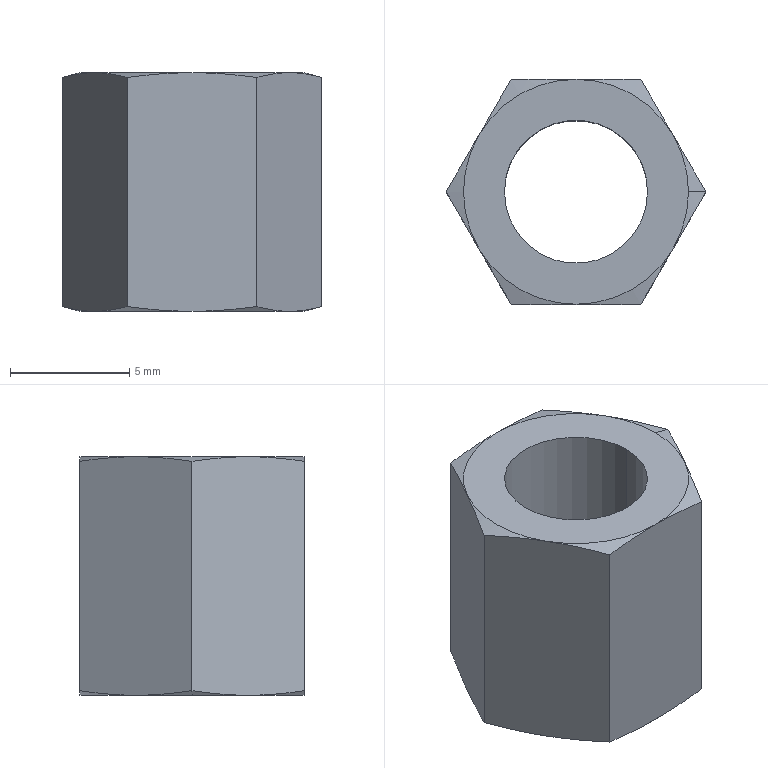Part | SolidWorks | features Cut 2, Chamfer 1, Extrusion 1, MoveFace 1 | 1 solid | 24 faces | box 10.89 x 9.431 x 10 mm | volume 486.676 mm3 | cone 14 | plane 8 | cylinder 2 | commonest cylinder face diameters 6 x2
STEP:
#1=CARTESIAN_POINT('',(4.716,0.,6.4));
#2=VERTEX_POINT('',#1);
#3=CARTESIAN_POINT('',(4.084,2.358,6.4));
#4=VERTEX_POINT('',#3);
#5=CARTESIAN_POINT('',(0.,0.,6.4));
#6=DIRECTION('',(0.,0.,1.));
#7=DIRECTION('',(1.,0.,0.));
#8=AXIS2_PLACEMENT_3D('',#5,#6,#7);
#9=CIRCLE('',#8,4.716);
#10=EDGE_CURVE('',#2,#4,#9,.T.);
#11=ORIENTED_EDGE('',*,*,#10,.F.);
#12=CARTESIAN_POINT('',(5.445,0.,6.205));
#13=VERTEX_POINT('',#12);
#14=CARTESIAN_POINT('',(4.716,0.,6.4));
#15=DIRECTION('',(0.9659,0.,-0.2588));
#16=VECTOR('',#15,1000.);
#17=LINE('',#14,#16);
#18=EDGE_CURVE('',#2,#13,#17,.T.);
#19=ORIENTED_EDGE('',*,*,#18,.T.);
#20=CARTESIAN_POINT('',(5.445,0.,6.205));
#21=CARTESIAN_POINT('',(4.991,0.7859,6.326));
#22=CARTESIAN_POINT('',(4.538,1.572,6.4));
#23=CARTESIAN_POINT('',(4.084,2.358,6.4));
#24=B_SPLINE_CURVE_WITH_KNOTS('',3,(#20,#21,#22,#23),.UNSPECIFIED.,.F.,.F.,(4,4),(0.000000231,0.002723),.UNSPECIFIED.);
#25=EDGE_CURVE('',#13,#4,#24,.T.);
#26=ORIENTED_EDGE('',*,*,#25,.T.);
#27=EDGE_LOOP('',(#11,#19,#26));
#28=FACE_OUTER_BOUND('',#27,.T.);
#29=CARTESIAN_POINT('',(0.,0.,6.4));
#30=DIRECTION('',(0.,0.,-1.));
#31=DIRECTION('',(1.,0.,0.));
#32=AXIS2_PLACEMENT_3D('',#29,#30,#31);
#33=CONICAL_SURFACE('',#32,4.716,1.309);
#34=ADVANCED_FACE('',(#28),#33,.T.);
#35=CARTESIAN_POINT('',(-4.716,0.,-3.6));
#36=VERTEX_POINT('',#35);
#37=CARTESIAN_POINT('',(-4.084,2.358,-3.6));
#38=VERTEX_POINT('',#37);
#39=CARTESIAN_POINT('',(0.,0.,-3.6));
#40=DIRECTION('',(0.,0.,-1.));
#41=DIRECTION('',(-1.,0.,0.));
#42=AXIS2_PLACEMENT_3D('',#39,#40,#41);
#43=CIRCLE('',#42,4.716);
#44=EDGE_CURVE('',#36,#38,#43,.T.);
#45=ORIENTED_EDGE('',*,*,#44,.F.);
#46=CARTESIAN_POINT('',(-5.445,0.,-3.405));
#47=VERTEX_POINT('',#46);
#48=CARTESIAN_POINT('',(-4.716,0.,-3.6));
#49=DIRECTION('',(-0.9659,0.,0.2588));
#50=VECTOR('',#49,1000.);
#51=LINE('',#48,#50);
#52=EDGE_CURVE('',#36,#47,#51,.T.);
#53=ORIENTED_EDGE('',*,*,#52,.T.);
#54=CARTESIAN_POINT('',(-5.445,0.,-3.405));
#55=CARTESIAN_POINT('',(-4.991,0.7861,-3.526));
#56=CARTESIAN_POINT('',(-4.537,1.572,-3.6));
#57=CARTESIAN_POINT('',(-4.084,2.358,-3.6));
#58=B_SPLINE_CURVE_WITH_KNOTS('',3,(#54,#55,#56,#57),.UNSPECIFIED.,.F.,.F.,(4,4),(0.02771,0.03044),.UNSPECIFIED.);
#59=EDGE_CURVE('',#47,#38,#58,.T.);
#60=ORIENTED_EDGE('',*,*,#59,.T.);
#61=EDGE_LOOP('',(#45,#53,#60));
#62=FACE_OUTER_BOUND('',#61,.T.);
#63=CARTESIAN_POINT('',(0.,0.,-3.6));
#64=DIRECTION('',(0.,0.,1.));
#65=DIRECTION('',(-1.,0.,0.));
#66=AXIS2_PLACEMENT_3D('',#63,#64,#65);
#67=CONICAL_SURFACE('',#66,4.716,1.309);
#68=ADVANCED_FACE('',(#62),#67,.T.);
#69=CARTESIAN_POINT('',(-3.,0.,6.4));
#70=VERTEX_POINT('',#69);
#71=CARTESIAN_POINT('',(3.,0.,6.4));
#72=VERTEX_POINT('',#71);
#73=CARTESIAN_POINT('',(0.,0.,6.4));
#74=DIRECTION('',(0.,0.,1.));
#75=DIRECTION('',(1.,0.,0.));
#76=AXIS2_PLACEMENT_3D('',#73,#74,#75);
#77=CIRCLE('',#76,3.);
#78=EDGE_CURVE('',#70,#72,#77,.T.);
#79=ORIENTED_EDGE('',*,*,#78,.T.);
#80=CARTESIAN_POINT('',(3.,0.,-3.6));
#81=VERTEX_POINT('',#80);
#82=CARTESIAN_POINT('',(3.,0.,6.4));
#83=DIRECTION('',(0.,0.,-1.));
#84=VECTOR('',#83,1000.);
#85=LINE('',#82,#84);
#86=EDGE_CURVE('',#72,#81,#85,.T.);
#87=ORIENTED_EDGE('',*,*,#86,.T.);
#88=CARTESIAN_POINT('',(-3.,0.,-3.6));
#89=VERTEX_POINT('',#88);
#90=CARTESIAN_POINT('',(0.,0.,-3.6));
#91=DIRECTION('',(0.,0.,1.));
#92=DIRECTION('',(1.,0.,0.));
#93=AXIS2_PLACEMENT_3D('',#90,#91,#92);
#94=CIRCLE('',#93,3.);
#95=EDGE_CURVE('',#89,#81,#94,.T.);
#96=ORIENTED_EDGE('',*,*,#95,.F.);
#97=CARTESIAN_POINT('',(-3.,0.,6.4));
#98=DIRECTION('',(0.,0.,-1.));
#99=VECTOR('',#98,1000.);
#100=LINE('',#97,#99);
#101=EDGE_CURVE('',#70,#89,#100,.T.);
#102=ORIENTED_EDGE('',*,*,#101,.F.);
#103=EDGE_LOOP('',(#79,#87,#96,#102));
#104=FACE_OUTER_BOUND('',#103,.T.);
#105=CARTESIAN_POINT('',(0.,0.,6.4));
#106=DIRECTION('',(0.,0.,-1.));
#107=DIRECTION('',(-1.,0.,0.));
#108=AXIS2_PLACEMENT_3D('',#105,#106,#107);
#109=CYLINDRICAL_SURFACE('',#108,3.);
#110=ADVANCED_FACE('',(#104),#109,.F.);
#111=ORIENTED_EDGE('',*,*,#25,.F.);
#112=CARTESIAN_POINT('',(5.445,0.,-3.405));
#113=VERTEX_POINT('',#112);
#114=CARTESIAN_POINT('',(5.445,0.,6.4));
#115=DIRECTION('',(0.,0.,-1.));
#116=VECTOR('',#115,1000.);
#117=LINE('',#114,#116);
#118=EDGE_CURVE('',#13,#113,#117,.T.);
#119=ORIENTED_EDGE('',*,*,#118,.T.);
#120=CARTESIAN_POINT('',(4.084,2.358,-3.6));
#121=VERTEX_POINT('',#120);
#122=CARTESIAN_POINT('',(4.084,2.358,-3.6));
#123=CARTESIAN_POINT('',(4.311,1.965,-3.6));
#124=CARTESIAN_POINT('',(4.539,1.569,-3.582));
#125=CARTESIAN_POINT('',(4.993,0.7831,-3.514));
#126=CARTESIAN_POINT('',(5.219,0.3911,-3.465));
#127=CARTESIAN_POINT('',(5.445,0.,-3.405));
#128=B_SPLINE_CURVE_WITH_KNOTS('',3,(#122,#123,#124,#125,#126,#127),.UNSPECIFIED.,.F.,.F.,(4,2,4),(0.02511,0.02644,0.02777),.UNSPECIFIED.);
#129=EDGE_CURVE('',#121,#113,#128,.T.);
#130=ORIENTED_EDGE('',*,*,#129,.F.);
#131=CARTESIAN_POINT('',(2.723,4.716,-3.405));
#132=VERTEX_POINT('',#131);
#133=CARTESIAN_POINT('',(2.723,4.716,-3.405));
#134=CARTESIAN_POINT('',(3.176,3.929,-3.526));
#135=CARTESIAN_POINT('',(3.63,3.143,-3.6));
#136=CARTESIAN_POINT('',(4.084,2.358,-3.6));
#137=B_SPLINE_CURVE_WITH_KNOTS('',3,(#133,#134,#135,#136),.UNSPECIFIED.,.F.,.F.,(4,4),(0.02771,0.03044),.UNSPECIFIED.);
#138=EDGE_CURVE('',#132,#121,#137,.T.);
#139=ORIENTED_EDGE('',*,*,#138,.F.);
#140=CARTESIAN_POINT('',(2.723,4.716,6.205));
#141=VERTEX_POINT('',#140);
#142=CARTESIAN_POINT('',(2.723,4.716,6.4));
#143=DIRECTION('',(0.,0.,-1.));
#144=VECTOR('',#143,1000.);
#145=LINE('',#142,#144);
#146=EDGE_CURVE('',#141,#132,#145,.T.);
#147=ORIENTED_EDGE('',*,*,#146,.F.);
#148=CARTESIAN_POINT('',(4.084,2.358,6.4));
#149=CARTESIAN_POINT('',(3.63,3.144,6.4));
#150=CARTESIAN_POINT('',(3.176,3.93,6.326));
#151=CARTESIAN_POINT('',(2.723,4.716,6.205));
#152=B_SPLINE_CURVE_WITH_KNOTS('',3,(#148,#149,#150,#151),.UNSPECIFIED.,.F.,.F.,(4,4),(0.002723,0.005445),.UNSPECIFIED.);
#153=EDGE_CURVE('',#4,#141,#152,.T.);
#154=ORIENTED_EDGE('',*,*,#153,.F.);
#155=EDGE_LOOP('',(#111,#119,#130,#139,#147,#154));
#156=FACE_OUTER_BOUND('',#155,.T.);
#157=CARTESIAN_POINT('',(5.445,0.,6.4));
#158=DIRECTION('',(-0.866,-0.5,0.));
#159=DIRECTION('',(0.5,-0.866,0.));
#160=AXIS2_PLACEMENT_3D('',#157,#158,#159);
#161=PLANE('',#160);
#162=ADVANCED_FACE('',(#156),#161,.F.);
#163=CARTESIAN_POINT('',(0.,4.716,6.4));
#164=VERTEX_POINT('',#163);
#165=CARTESIAN_POINT('',(2.723,4.716,6.205));
#166=CARTESIAN_POINT('',(1.816,4.716,6.326));
#167=CARTESIAN_POINT('',(0.9092,4.716,6.4));
#168=CARTESIAN_POINT('',(0.,4.716,6.4));
#169=B_SPLINE_CURVE_WITH_KNOTS('',3,(#165,#166,#167,#168),.UNSPECIFIED.,.F.,.F.,(4,4),(0.01615,0.01889),.UNSPECIFIED.);
#170=EDGE_CURVE('',#141,#164,#169,.T.);
#171=ORIENTED_EDGE('',*,*,#170,.F.);
#172=ORIENTED_EDGE('',*,*,#146,.T.);
#173=CARTESIAN_POINT('',(0.,4.716,-3.6));
#174=VERTEX_POINT('',#173);
#175=CARTESIAN_POINT('',(0.,4.716,-3.6));
#176=CARTESIAN_POINT('',(0.454,4.716,-3.6));
#177=CARTESIAN_POINT('',(0.9107,4.716,-3.582));
#178=CARTESIAN_POINT('',(1.818,4.716,-3.514));
#179=CARTESIAN_POINT('',(2.271,4.716,-3.465));
#180=CARTESIAN_POINT('',(2.723,4.716,-3.405));
#181=B_SPLINE_CURVE_WITH_KNOTS('',3,(#175,#176,#177,#178,#179,#180),.UNSPECIFIED.,.F.,.F.,(4,2,4),(0.02511,0.02644,0.02777),.UNSPECIFIED.);
#182=EDGE_CURVE('',#174,#132,#181,.T.);
#183=ORIENTED_EDGE('',*,*,#182,.F.);
#184=CARTESIAN_POINT('',(-2.722,4.716,-3.405));
#185=VERTEX_POINT('',#184);
#186=CARTESIAN_POINT('',(-2.722,4.716,-3.405));
#187=CARTESIAN_POINT('',(-1.815,4.716,-3.526));
#188=CARTESIAN_POINT('',(-0.9073,4.716,-3.6));
#189=CARTESIAN_POINT('',(0.,4.716,-3.6));
#190=B_SPLINE_CURVE_WITH_KNOTS('',3,(#186,#187,#188,#189),.UNSPECIFIED.,.F.,.F.,(4,4),(0.02771,0.03044),.UNSPECIFIED.);
#191=EDGE_CURVE('',#185,#174,#190,.T.);
#192=ORIENTED_EDGE('',*,*,#191,.F.);
#193=CARTESIAN_POINT('',(-2.722,4.716,6.205));
#194=VERTEX_POINT('',#193);
#195=CARTESIAN_POINT('',(-2.722,4.716,6.4));
#196=DIRECTION('',(0.,0.,-1.));
#197=VECTOR('',#196,1000.);
#198=LINE('',#195,#197);
#199=EDGE_CURVE('',#194,#185,#198,.T.);
#200=ORIENTED_EDGE('',*,*,#199,.F.);
#201=CARTESIAN_POINT('',(0.,4.716,6.4));
#202=CARTESIAN_POINT('',(-0.4531,4.716,6.4));
#203=CARTESIAN_POINT('',(-0.9068,4.716,6.382));
#204=CARTESIAN_POINT('',(-1.815,4.716,6.315));
#205=CARTESIAN_POINT('',(-2.27,4.716,6.265));
#206=CARTESIAN_POINT('',(-2.722,4.716,6.205));
#207=B_SPLINE_CURVE_WITH_KNOTS('',3,(#201,#202,#203,#204,#205,#206),.UNSPECIFIED.,.F.,.F.,(4,2,4),(0.01889,0.02026,0.02162),.UNSPECIFIED.);
#208=EDGE_CURVE('',#164,#194,#207,.T.);
#209=ORIENTED_EDGE('',*,*,#208,.F.);
#210=EDGE_LOOP('',(#171,#172,#183,#192,#200,#209));
#211=FACE_OUTER_BOUND('',#210,.T.);
#212=CARTESIAN_POINT('',(2.723,4.716,6.4));
#213=DIRECTION('',(0.,-1.,0.));
#214=DIRECTION('',(0.,0.,-1.));
#215=AXIS2_PLACEMENT_3D('',#212,#213,#214);
#216=PLANE('',#215);
#217=ADVANCED_FACE('',(#211),#216,.F.);
#218=CARTESIAN_POINT('',(-4.084,2.358,6.4));
#219=VERTEX_POINT('',#218);
#220=CARTESIAN_POINT('',(-2.722,4.716,6.205));
#221=CARTESIAN_POINT('',(-3.176,3.93,6.326));
#222=CARTESIAN_POINT('',(-3.63,3.144,6.4));
#223=CARTESIAN_POINT('',(-4.084,2.358,6.4));
#224=B_SPLINE_CURVE_WITH_KNOTS('',3,(#220,#221,#222,#223),.UNSPECIFIED.,.F.,.F.,(4,4),(0.000000231,0.002723),.UNSPECIFIED.);
#225=EDGE_CURVE('',#194,#219,#224,.T.);
#226=ORIENTED_EDGE('',*,*,#225,.F.);
#227=ORIENTED_EDGE('',*,*,#199,.T.);
#228=CARTESIAN_POINT('',(-4.084,2.358,-3.6));
#229=CARTESIAN_POINT('',(-3.857,2.751,-3.6));
#230=CARTESIAN_POINT('',(-3.628,3.146,-3.582));
#231=CARTESIAN_POINT('',(-3.175,3.932,-3.514));
#232=CARTESIAN_POINT('',(-2.948,4.324,-3.465));
#233=CARTESIAN_POINT('',(-2.722,4.716,-3.405));
#234=B_SPLINE_CURVE_WITH_KNOTS('',3,(#228,#229,#230,#231,#232,#233),.UNSPECIFIED.,.F.,.F.,(4,2,4),(0.02511,0.02644,0.02777),.UNSPECIFIED.);
#235=EDGE_CURVE('',#38,#185,#234,.T.);
#236=ORIENTED_EDGE('',*,*,#235,.F.);
#237=ORIENTED_EDGE('',*,*,#59,.F.);
#238=CARTESIAN_POINT('',(-5.445,0.,6.205));
#239=VERTEX_POINT('',#238);
#240=CARTESIAN_POINT('',(-5.445,0.,6.4));
#241=DIRECTION('',(0.,0.,-1.));
#242=VECTOR('',#241,1000.);
#243=LINE('',#240,#242);
#244=EDGE_CURVE('',#239,#47,#243,.T.);
#245=ORIENTED_EDGE('',*,*,#244,.F.);
#246=CARTESIAN_POINT('',(-4.084,2.358,6.4));
#247=CARTESIAN_POINT('',(-4.537,1.572,6.4));
#248=CARTESIAN_POINT('',(-4.991,0.7859,6.326));
#249=CARTESIAN_POINT('',(-5.445,0.,6.205));
#250=B_SPLINE_CURVE_WITH_KNOTS('',3,(#246,#247,#248,#249),.UNSPECIFIED.,.F.,.F.,(4,4),(0.002723,0.005445),.UNSPECIFIED.);
#251=EDGE_CURVE('',#219,#239,#250,.T.);
#252=ORIENTED_EDGE('',*,*,#251,.F.);
#253=EDGE_LOOP('',(#226,#227,#236,#237,#245,#252));
#254=FACE_OUTER_BOUND('',#253,.T.);
#255=CARTESIAN_POINT('',(-2.722,4.716,6.4));
#256=DIRECTION('',(0.866,-0.5,0.));
#257=DIRECTION('',(0.5,0.866,0.));
#258=AXIS2_PLACEMENT_3D('',#255,#256,#257);
#259=PLANE('',#258);
#260=ADVANCED_FACE('',(#254),#259,.F.);
#261=CARTESIAN_POINT('',(-4.084,-2.358,6.4));
#262=VERTEX_POINT('',#261);
#263=CARTESIAN_POINT('',(-5.445,0.,6.205));
#264=CARTESIAN_POINT('',(-4.991,-0.7859,6.326));
#265=CARTESIAN_POINT('',(-4.537,-1.572,6.4));
#266=CARTESIAN_POINT('',(-4.084,-2.358,6.4));
#267=B_SPLINE_CURVE_WITH_KNOTS('',3,(#263,#264,#265,#266),.UNSPECIFIED.,.F.,.F.,(4,4),(0.000000231,0.002723),.UNSPECIFIED.);
#268=EDGE_CURVE('',#239,#262,#267,.T.);
#269=ORIENTED_EDGE('',*,*,#268,.F.);
#270=ORIENTED_EDGE('',*,*,#244,.T.);
#271=CARTESIAN_POINT('',(-4.084,-2.358,-3.6));
#272=VERTEX_POINT('',#271);
#273=CARTESIAN_POINT('',(-4.084,-2.358,-3.6));
#274=CARTESIAN_POINT('',(-4.311,-1.965,-3.6));
#275=CARTESIAN_POINT('',(-4.539,-1.569,-3.582));
#276=CARTESIAN_POINT('',(-4.993,-0.7831,-3.514));
#277=CARTESIAN_POINT('',(-5.219,-0.3911,-3.465));
#278=CARTESIAN_POINT('',(-5.445,0.,-3.405));
#279=B_SPLINE_CURVE_WITH_KNOTS('',3,(#273,#274,#275,#276,#277,#278),.UNSPECIFIED.,.F.,.F.,(4,2,4),(0.02511,0.02644,0.02777),.UNSPECIFIED.);
#280=EDGE_CURVE('',#272,#47,#279,.T.);
#281=ORIENTED_EDGE('',*,*,#280,.F.);
#282=CARTESIAN_POINT('',(-2.722,-4.716,-3.405));
#283=VERTEX_POINT('',#282);
#284=CARTESIAN_POINT('',(-2.722,-4.716,-3.405));
#285=CARTESIAN_POINT('',(-3.176,-3.929,-3.526));
#286=CARTESIAN_POINT('',(-3.63,-3.143,-3.6));
#287=CARTESIAN_POINT('',(-4.084,-2.358,-3.6));
#288=B_SPLINE_CURVE_WITH_KNOTS('',3,(#284,#285,#286,#287),.UNSPECIFIED.,.F.,.F.,(4,4),(0.02771,0.03044),.UNSPECIFIED.);
#289=EDGE_CURVE('',#283,#272,#288,.T.);
#290=ORIENTED_EDGE('',*,*,#289,.F.);
#291=CARTESIAN_POINT('',(-2.722,-4.716,6.205));
#292=VERTEX_POINT('',#291);
#293=CARTESIAN_POINT('',(-2.722,-4.716,6.4));
#294=DIRECTION('',(0.,0.,-1.));
#295=VECTOR('',#294,1000.);
#296=LINE('',#293,#295);
#297=EDGE_CURVE('',#292,#283,#296,.T.);
#298=ORIENTED_EDGE('',*,*,#297,.F.);
#299=CARTESIAN_POINT('',(-4.084,-2.358,6.4));
#300=CARTESIAN_POINT('',(-3.63,-3.144,6.4));
#301=CARTESIAN_POINT('',(-3.176,-3.93,6.326));
#302=CARTESIAN_POINT('',(-2.722,-4.716,6.205));
#303=B_SPLINE_CURVE_WITH_KNOTS('',3,(#299,#300,#301,#302),.UNSPECIFIED.,.F.,.F.,(4,4),(0.002723,0.005445),.UNSPECIFIED.);
#304=EDGE_CURVE('',#262,#292,#303,.T.);
#305=ORIENTED_EDGE('',*,*,#304,.F.);
#306=EDGE_LOOP('',(#269,#270,#281,#290,#298,#305));
#307=FACE_OUTER_BOUND('',#306,.T.);
#308=CARTESIAN_POINT('',(-5.445,0.,6.4));
#309=DIRECTION('',(0.866,0.5,0.));
#310=DIRECTION('',(-0.5,0.866,0.));
#311=AXIS2_PLACEMENT_3D('',#308,#309,#310);
#312=PLANE('',#311);
#313=ADVANCED_FACE('',(#307),#312,.F.);
#314=CARTESIAN_POINT('',(0.,-4.716,6.4));
#315=VERTEX_POINT('',#314);
#316=CARTESIAN_POINT('',(-2.722,-4.716,6.205));
#317=CARTESIAN_POINT('',(-2.27,-4.716,6.265));
#318=CARTESIAN_POINT('',(-1.815,-4.716,6.315));
#319=CARTESIAN_POINT('',(-0.9068,-4.716,6.382));
#320=CARTESIAN_POINT('',(-0.4531,-4.716,6.4));
#321=CARTESIAN_POINT('',(0.,-4.716,6.4));
#322=B_SPLINE_CURVE_WITH_KNOTS('',3,(#316,#317,#318,#319,#320,#321),.UNSPECIFIED.,.F.,.F.,(4,2,4),(0.004659,0.006027,0.007395),.UNSPECIFIED.);
#323=EDGE_CURVE('',#292,#315,#322,.T.);
#324=ORIENTED_EDGE('',*,*,#323,.F.);
#325=ORIENTED_EDGE('',*,*,#297,.T.);
#326=CARTESIAN_POINT('',(0.,-4.716,-3.6));
#327=VERTEX_POINT('',#326);
#328=CARTESIAN_POINT('',(0.,-4.716,-3.6));
#329=CARTESIAN_POINT('',(-0.454,-4.716,-3.6));
#330=CARTESIAN_POINT('',(-0.9107,-4.716,-3.582));
#331=CARTESIAN_POINT('',(-1.818,-4.716,-3.514));
#332=CARTESIAN_POINT('',(-2.271,-4.716,-3.465));
#333=CARTESIAN_POINT('',(-2.722,-4.716,-3.405));
#334=B_SPLINE_CURVE_WITH_KNOTS('',3,(#328,#329,#330,#331,#332,#333),.UNSPECIFIED.,.F.,.F.,(4,2,4),(0.02511,0.02644,0.02777),.UNSPECIFIED.);
#335=EDGE_CURVE('',#327,#283,#334,.T.);
#336=ORIENTED_EDGE('',*,*,#335,.F.);
#337=CARTESIAN_POINT('',(2.723,-4.716,-3.405));
#338=VERTEX_POINT('',#337);
#339=CARTESIAN_POINT('',(2.723,-4.716,-3.405));
#340=CARTESIAN_POINT('',(1.815,-4.716,-3.526));
#341=CARTESIAN_POINT('',(0.9073,-4.716,-3.6));
#342=CARTESIAN_POINT('',(0.,-4.716,-3.6));
#343=B_SPLINE_CURVE_WITH_KNOTS('',3,(#339,#340,#341,#342),.UNSPECIFIED.,.F.,.F.,(4,4),(0.02771,0.03044),.UNSPECIFIED.);
#344=EDGE_CURVE('',#338,#327,#343,.T.);
#345=ORIENTED_EDGE('',*,*,#344,.F.);
#346=CARTESIAN_POINT('',(2.723,-4.716,6.205));
#347=VERTEX_POINT('',#346);
#348=CARTESIAN_POINT('',(2.723,-4.716,6.4));
#349=DIRECTION('',(0.,0.,-1.));
#350=VECTOR('',#349,1000.);
#351=LINE('',#348,#350);
#352=EDGE_CURVE('',#347,#338,#351,.T.);
#353=ORIENTED_EDGE('',*,*,#352,.F.);
#354=CARTESIAN_POINT('',(0.,-4.716,6.4));
#355=CARTESIAN_POINT('',(0.9092,-4.716,6.4));
#356=CARTESIAN_POINT('',(1.816,-4.716,6.326));
#357=CARTESIAN_POINT('',(2.723,-4.716,6.205));
#358=B_SPLINE_CURVE_WITH_KNOTS('',3,(#354,#355,#356,#357),.UNSPECIFIED.,.F.,.F.,(4,4),(0.007395,0.01014),.UNSPECIFIED.);
#359=EDGE_CURVE('',#315,#347,#358,.T.);
#360=ORIENTED_EDGE('',*,*,#359,.F.);
#361=EDGE_LOOP('',(#324,#325,#336,#345,#353,#360));
#362=FACE_OUTER_BOUND('',#361,.T.);
#363=CARTESIAN_POINT('',(-2.722,-4.716,6.4));
#364=DIRECTION('',(0.,1.,0.));
#365=DIRECTION('',(0.,0.,1.));
#366=AXIS2_PLACEMENT_3D('',#363,#364,#365);
#367=PLANE('',#366);
#368=ADVANCED_FACE('',(#362),#367,.F.);
#369=CARTESIAN_POINT('',(4.084,-2.358,6.4));
#370=VERTEX_POINT('',#369);
#371=CARTESIAN_POINT('',(2.723,-4.716,6.205));
#372=CARTESIAN_POINT('',(3.176,-3.93,6.326));
#373=CARTESIAN_POINT('',(3.63,-3.144,6.4));
#374=CARTESIAN_POINT('',(4.084,-2.358,6.4));
#375=B_SPLINE_CURVE_WITH_KNOTS('',3,(#371,#372,#373,#374),.UNSPECIFIED.,.F.,.F.,(4,4),(0.000000231,0.002723),.UNSPECIFIED.);
#376=EDGE_CURVE('',#347,#370,#375,.T.);
#377=ORIENTED_EDGE('',*,*,#376,.F.);
#378=ORIENTED_EDGE('',*,*,#352,.T.);
#379=CARTESIAN_POINT('',(4.084,-2.358,-3.6));
#380=VERTEX_POINT('',#379);
#381=CARTESIAN_POINT('',(4.084,-2.358,-3.6));
#382=CARTESIAN_POINT('',(3.857,-2.751,-3.6));
#383=CARTESIAN_POINT('',(3.628,-3.146,-3.582));
#384=CARTESIAN_POINT('',(3.175,-3.932,-3.514));
#385=CARTESIAN_POINT('',(2.948,-4.324,-3.465));
#386=CARTESIAN_POINT('',(2.723,-4.716,-3.405));
#387=B_SPLINE_CURVE_WITH_KNOTS('',3,(#381,#382,#383,#384,#385,#386),.UNSPECIFIED.,.F.,.F.,(4,2,4),(0.02511,0.02644,0.02777),.UNSPECIFIED.);
#388=EDGE_CURVE('',#380,#338,#387,.T.);
#389=ORIENTED_EDGE('',*,*,#388,.F.);
#390=CARTESIAN_POINT('',(5.445,0.,-3.405));
#391=CARTESIAN_POINT('',(4.991,-0.7861,-3.526));
#392=CARTESIAN_POINT('',(4.537,-1.572,-3.6));
#393=CARTESIAN_POINT('',(4.084,-2.358,-3.6));
#394=B_SPLINE_CURVE_WITH_KNOTS('',3,(#390,#391,#392,#393),.UNSPECIFIED.,.F.,.F.,(4,4),(0.02771,0.03044),.UNSPECIFIED.);
#395=EDGE_CURVE('',#113,#380,#394,.T.);
#396=ORIENTED_EDGE('',*,*,#395,.F.);
#397=ORIENTED_EDGE('',*,*,#118,.F.);
#398=CARTESIAN_POINT('',(4.084,-2.358,6.4));
#399=CARTESIAN_POINT('',(4.538,-1.572,6.4));
#400=CARTESIAN_POINT('',(4.991,-0.7859,6.326));
#401=CARTESIAN_POINT('',(5.445,0.,6.205));
#402=B_SPLINE_CURVE_WITH_KNOTS('',3,(#398,#399,#400,#401),.UNSPECIFIED.,.F.,.F.,(4,4),(0.002723,0.005445),.UNSPECIFIED.);
#403=EDGE_CURVE('',#370,#13,#402,.T.);
#404=ORIENTED_EDGE('',*,*,#403,.F.);
#405=EDGE_LOOP('',(#377,#378,#389,#396,#397,#404));
#406=FACE_OUTER_BOUND('',#405,.T.);
#407=CARTESIAN_POINT('',(2.723,-4.716,6.4));
#408=DIRECTION('',(-0.866,0.5,0.));
#409=DIRECTION('',(-0.5,-0.866,0.));
#410=AXIS2_PLACEMENT_3D('',#407,#408,#409);
#411=PLANE('',#410);
#412=ADVANCED_FACE('',(#406),#411,.F.);
#413=ORIENTED_EDGE('',*,*,#78,.F.);
#414=CARTESIAN_POINT('',(0.,0.,6.4));
#415=DIRECTION('',(0.,0.,1.));
#416=DIRECTION('',(1.,0.,0.));
#417=AXIS2_PLACEMENT_3D('',#414,#415,#416);
#418=CIRCLE('',#417,3.);
#419=EDGE_CURVE('',#72,#70,#418,.T.);
#420=ORIENTED_EDGE('',*,*,#419,.F.);
#421=EDGE_LOOP('',(#413,#420));
#422=FACE_BOUND('',#421,.T.);
#423=CARTESIAN_POINT('',(0.,0.,6.4));
#424=DIRECTION('',(0.,0.,1.));
#425=DIRECTION('',(1.,0.,0.));
#426=AXIS2_PLACEMENT_3D('',#423,#424,#425);
#427=CIRCLE('',#426,4.716);
#428=EDGE_CURVE('',#370,#2,#427,.T.);
#429=ORIENTED_EDGE('',*,*,#428,.T.);
#430=ORIENTED_EDGE('',*,*,#10,.T.);
#431=CARTESIAN_POINT('',(0.,0.,6.4));
#432=DIRECTION('',(0.,0.,1.));
#433=DIRECTION('',(1.,0.,0.));
#434=AXIS2_PLACEMENT_3D('',#431,#432,#433);
#435=CIRCLE('',#434,4.716);
#436=EDGE_CURVE('',#4,#164,#435,.T.);
#437=ORIENTED_EDGE('',*,*,#436,.T.);
#438=CARTESIAN_POINT('',(0.,0.,6.4));
#439=DIRECTION('',(0.,0.,1.));
#440=DIRECTION('',(1.,0.,0.));
#441=AXIS2_PLACEMENT_3D('',#438,#439,#440);
#442=CIRCLE('',#441,4.716);
#443=EDGE_CURVE('',#164,#219,#442,.T.);
#444=ORIENTED_EDGE('',*,*,#443,.T.);
#445=CARTESIAN_POINT('',(0.,0.,6.4));
#446=DIRECTION('',(0.,0.,1.));
#447=DIRECTION('',(1.,0.,0.));
#448=AXIS2_PLACEMENT_3D('',#445,#446,#447);
#449=CIRCLE('',#448,4.716);
#450=EDGE_CURVE('',#219,#262,#449,.T.);
#451=ORIENTED_EDGE('',*,*,#450,.T.);
#452=CARTESIAN_POINT('',(0.,0.,6.4));
#453=DIRECTION('',(0.,0.,1.));
#454=DIRECTION('',(1.,0.,0.));
#455=AXIS2_PLACEMENT_3D('',#452,#453,#454);
#456=CIRCLE('',#455,4.716);
#457=EDGE_CURVE('',#262,#315,#456,.T.);
#458=ORIENTED_EDGE('',*,*,#457,.T.);
#459=CARTESIAN_POINT('',(0.,0.,6.4));
#460=DIRECTION('',(0.,0.,1.));
#461=DIRECTION('',(1.,0.,0.));
#462=AXIS2_PLACEMENT_3D('',#459,#460,#461);
#463=CIRCLE('',#462,4.716);
#464=EDGE_CURVE('',#315,#370,#463,.T.);
#465=ORIENTED_EDGE('',*,*,#464,.T.);
#466=EDGE_LOOP('',(#429,#430,#437,#444,#451,#458,#465));
#467=FACE_OUTER_BOUND('',#466,.T.);
#468=CARTESIAN_POINT('',(2.723,4.716,6.4));
#469=DIRECTION('',(0.,0.,1.));
#470=DIRECTION('',(1.,0.,0.));
#471=AXIS2_PLACEMENT_3D('',#468,#469,#470);
#472=PLANE('',#471);
#473=ADVANCED_FACE('',(#422,#467),#472,.T.);
#474=ORIENTED_EDGE('',*,*,#95,.T.);
#475=CARTESIAN_POINT('',(0.,0.,-3.6));
#476=DIRECTION('',(0.,0.,1.));
#477=DIRECTION('',(1.,0.,0.));
#478=AXIS2_PLACEMENT_3D('',#475,#476,#477);
#479=CIRCLE('',#478,3.);
#480=EDGE_CURVE('',#81,#89,#479,.T.);
#481=ORIENTED_EDGE('',*,*,#480,.T.);
#482=EDGE_LOOP('',(#474,#481));
#483=FACE_BOUND('',#482,.T.);
#484=CARTESIAN_POINT('',(0.,0.,-3.6));
#485=DIRECTION('',(0.,0.,-1.));
#486=DIRECTION('',(-1.,0.,0.));
#487=AXIS2_PLACEMENT_3D('',#484,#485,#486);
#488=CIRCLE('',#487,4.716);
#489=EDGE_CURVE('',#174,#121,#488,.T.);
#490=ORIENTED_EDGE('',*,*,#489,.T.);
#491=CARTESIAN_POINT('',(0.,0.,-3.6));
#492=DIRECTION('',(0.,0.,-1.));
#493=DIRECTION('',(-1.,0.,0.));
#494=AXIS2_PLACEMENT_3D('',#491,#492,#493);
#495=CIRCLE('',#494,4.716);
#496=EDGE_CURVE('',#121,#380,#495,.T.);
#497=ORIENTED_EDGE('',*,*,#496,.T.);
#498=CARTESIAN_POINT('',(0.,0.,-3.6));
#499=DIRECTION('',(0.,0.,-1.));
#500=DIRECTION('',(-1.,0.,0.));
#501=AXIS2_PLACEMENT_3D('',#498,#499,#500);
#502=CIRCLE('',#501,4.716);
#503=EDGE_CURVE('',#380,#327,#502,.T.);
#504=ORIENTED_EDGE('',*,*,#503,.T.);
#505=CARTESIAN_POINT('',(0.,0.,-3.6));
#506=DIRECTION('',(0.,0.,-1.));
#507=DIRECTION('',(-1.,0.,0.));
#508=AXIS2_PLACEMENT_3D('',#505,#506,#507);
#509=CIRCLE('',#508,4.716);
#510=EDGE_CURVE('',#327,#272,#509,.T.);
#511=ORIENTED_EDGE('',*,*,#510,.T.);
#512=CARTESIAN_POINT('',(0.,0.,-3.6));
#513=DIRECTION('',(0.,0.,-1.));
#514=DIRECTION('',(-1.,0.,0.));
#515=AXIS2_PLACEMENT_3D('',#512,#513,#514);
#516=CIRCLE('',#515,4.716);
#517=EDGE_CURVE('',#272,#36,#516,.T.);
#518=ORIENTED_EDGE('',*,*,#517,.T.);
#519=ORIENTED_EDGE('',*,*,#44,.T.);
#520=CARTESIAN_POINT('',(0.,0.,-3.6));
#521=DIRECTION('',(0.,0.,-1.));
#522=DIRECTION('',(-1.,0.,0.));
#523=AXIS2_PLACEMENT_3D('',#520,#521,#522);
#524=CIRCLE('',#523,4.716);
#525=EDGE_CURVE('',#38,#174,#524,.T.);
#526=ORIENTED_EDGE('',*,*,#525,.T.);
#527=EDGE_LOOP('',(#490,#497,#504,#511,#518,#519,#526));
#528=FACE_OUTER_BOUND('',#527,.T.);
#529=CARTESIAN_POINT('',(2.723,4.716,-3.6));
#530=DIRECTION('',(0.,0.,1.));
#531=DIRECTION('',(1.,0.,0.));
#532=AXIS2_PLACEMENT_3D('',#529,#530,#531);
#533=PLANE('',#532);
#534=ADVANCED_FACE('',(#483,#528),#533,.F.);
#535=ORIENTED_EDGE('',*,*,#86,.F.);
#536=ORIENTED_EDGE('',*,*,#419,.T.);
#537=ORIENTED_EDGE('',*,*,#101,.T.);
#538=ORIENTED_EDGE('',*,*,#480,.F.);
#539=EDGE_LOOP('',(#535,#536,#537,#538));
#540=FACE_OUTER_BOUND('',#539,.T.);
#541=CARTESIAN_POINT('',(0.,0.,6.4));
#542=DIRECTION('',(0.,0.,-1.));
#543=DIRECTION('',(-1.,0.,0.));
#544=AXIS2_PLACEMENT_3D('',#541,#542,#543);
#545=CYLINDRICAL_SURFACE('',#544,3.);
#546=ADVANCED_FACE('',(#540),#545,.F.);
#547=ORIENTED_EDGE('',*,*,#344,.T.);
#548=ORIENTED_EDGE('',*,*,#503,.F.);
#549=ORIENTED_EDGE('',*,*,#388,.T.);
#550=EDGE_LOOP('',(#547,#548,#549));
#551=FACE_OUTER_BOUND('',#550,.T.);
#552=CARTESIAN_POINT('',(0.,0.,-3.6));
#553=DIRECTION('',(0.,0.,1.));
#554=DIRECTION('',(-1.,0.,0.));
#555=AXIS2_PLACEMENT_3D('',#552,#553,#554);
#556=CONICAL_SURFACE('',#555,4.716,1.309);
#557=ADVANCED_FACE('',(#551),#556,.T.);
#558=ORIENTED_EDGE('',*,*,#129,.T.);
#559=ORIENTED_EDGE('',*,*,#395,.T.);
#560=ORIENTED_EDGE('',*,*,#496,.F.);
#561=EDGE_LOOP('',(#558,#559,#560));
#562=FACE_OUTER_BOUND('',#561,.T.);
#563=CARTESIAN_POINT('',(0.,0.,-3.6));
#564=DIRECTION('',(0.,0.,1.));
#565=DIRECTION('',(-1.,0.,0.));
#566=AXIS2_PLACEMENT_3D('',#563,#564,#565);
#567=CONICAL_SURFACE('',#566,4.716,1.309);
#568=ADVANCED_FACE('',(#562),#567,.T.);
#569=ORIENTED_EDGE('',*,*,#289,.T.);
#570=ORIENTED_EDGE('',*,*,#510,.F.);
#571=ORIENTED_EDGE('',*,*,#335,.T.);
#572=EDGE_LOOP('',(#569,#570,#571));
#573=FACE_OUTER_BOUND('',#572,.T.);
#574=CARTESIAN_POINT('',(0.,0.,-3.6));
#575=DIRECTION('',(0.,0.,1.));
#576=DIRECTION('',(-1.,0.,0.));
#577=AXIS2_PLACEMENT_3D('',#574,#575,#576);
#578=CONICAL_SURFACE('',#577,4.716,1.309);
#579=ADVANCED_FACE('',(#573),#578,.T.);
#580=ORIENTED_EDGE('',*,*,#52,.F.);
#581=ORIENTED_EDGE('',*,*,#517,.F.);
#582=ORIENTED_EDGE('',*,*,#280,.T.);
#583=EDGE_LOOP('',(#580,#581,#582));
#584=FACE_OUTER_BOUND('',#583,.T.);
#585=CARTESIAN_POINT('',(0.,0.,-3.6));
#586=DIRECTION('',(0.,0.,1.));
#587=DIRECTION('',(-1.,0.,0.));
#588=AXIS2_PLACEMENT_3D('',#585,#586,#587);
#589=CONICAL_SURFACE('',#588,4.716,1.309);
#590=ADVANCED_FACE('',(#584),#589,.T.);
#591=ORIENTED_EDGE('',*,*,#235,.T.);
#592=ORIENTED_EDGE('',*,*,#191,.T.);
#593=ORIENTED_EDGE('',*,*,#525,.F.);
#594=EDGE_LOOP('',(#591,#592,#593));
#595=FACE_OUTER_BOUND('',#594,.T.);
#596=CARTESIAN_POINT('',(0.,0.,-3.6));
#597=DIRECTION('',(0.,0.,1.));
#598=DIRECTION('',(-1.,0.,0.));
#599=AXIS2_PLACEMENT_3D('',#596,#597,#598);
#600=CONICAL_SURFACE('',#599,4.716,1.309);
#601=ADVANCED_FACE('',(#595),#600,.T.);
#602=ORIENTED_EDGE('',*,*,#182,.T.);
#603=ORIENTED_EDGE('',*,*,#138,.T.);
#604=ORIENTED_EDGE('',*,*,#489,.F.);
#605=EDGE_LOOP('',(#602,#603,#604));
#606=FACE_OUTER_BOUND('',#605,.T.);
#607=CARTESIAN_POINT('',(0.,0.,-3.6));
#608=DIRECTION('',(0.,0.,1.));
#609=DIRECTION('',(-1.,0.,0.));
#610=AXIS2_PLACEMENT_3D('',#607,#608,#609);
#611=CONICAL_SURFACE('',#610,4.716,1.309);
#612=ADVANCED_FACE('',(#606),#611,.T.);
#613=ORIENTED_EDGE('',*,*,#18,.F.);
#614=ORIENTED_EDGE('',*,*,#428,.F.);
#615=ORIENTED_EDGE('',*,*,#403,.T.);
#616=EDGE_LOOP('',(#613,#614,#615));
#617=FACE_OUTER_BOUND('',#616,.T.);
#618=CARTESIAN_POINT('',(0.,0.,6.4));
#619=DIRECTION('',(0.,0.,-1.));
#620=DIRECTION('',(1.,0.,0.));
#621=AXIS2_PLACEMENT_3D('',#618,#619,#620);
#622=CONICAL_SURFACE('',#621,4.716,1.309);
#623=ADVANCED_FACE('',(#617),#622,.T.);
#624=ORIENTED_EDGE('',*,*,#359,.T.);
#625=ORIENTED_EDGE('',*,*,#376,.T.);
#626=ORIENTED_EDGE('',*,*,#464,.F.);
#627=EDGE_LOOP('',(#624,#625,#626));
#628=FACE_OUTER_BOUND('',#627,.T.);
#629=CARTESIAN_POINT('',(0.,0.,6.4));
#630=DIRECTION('',(0.,0.,-1.));
#631=DIRECTION('',(1.,0.,0.));
#632=AXIS2_PLACEMENT_3D('',#629,#630,#631);
#633=CONICAL_SURFACE('',#632,4.716,1.309);
#634=ADVANCED_FACE('',(#628),#633,.T.);
#635=ORIENTED_EDGE('',*,*,#304,.T.);
#636=ORIENTED_EDGE('',*,*,#323,.T.);
#637=ORIENTED_EDGE('',*,*,#457,.F.);
#638=EDGE_LOOP('',(#635,#636,#637));
#639=FACE_OUTER_BOUND('',#638,.T.);
#640=CARTESIAN_POINT('',(0.,0.,6.4));
#641=DIRECTION('',(0.,0.,-1.));
#642=DIRECTION('',(1.,0.,0.));
#643=AXIS2_PLACEMENT_3D('',#640,#641,#642);
#644=CONICAL_SURFACE('',#643,4.716,1.309);
#645=ADVANCED_FACE('',(#639),#644,.T.);
#646=ORIENTED_EDGE('',*,*,#251,.T.);
#647=ORIENTED_EDGE('',*,*,#268,.T.);
#648=ORIENTED_EDGE('',*,*,#450,.F.);
#649=EDGE_LOOP('',(#646,#647,#648));
#650=FACE_OUTER_BOUND('',#649,.T.);
#651=CARTESIAN_POINT('',(0.,0.,6.4));
#652=DIRECTION('',(0.,0.,-1.));
#653=DIRECTION('',(1.,0.,0.));
#654=AXIS2_PLACEMENT_3D('',#651,#652,#653);
#655=CONICAL_SURFACE('',#654,4.716,1.309);
#656=ADVANCED_FACE('',(#650),#655,.T.);
#657=ORIENTED_EDGE('',*,*,#208,.T.);
#658=ORIENTED_EDGE('',*,*,#225,.T.);
#659=ORIENTED_EDGE('',*,*,#443,.F.);
#660=EDGE_LOOP('',(#657,#658,#659));
#661=FACE_OUTER_BOUND('',#660,.T.);
#662=CARTESIAN_POINT('',(0.,0.,6.4));
#663=DIRECTION('',(0.,0.,-1.));
#664=DIRECTION('',(1.,0.,0.));
#665=AXIS2_PLACEMENT_3D('',#662,#663,#664);
#666=CONICAL_SURFACE('',#665,4.716,1.309);
#667=ADVANCED_FACE('',(#661),#666,.T.);
#668=ORIENTED_EDGE('',*,*,#153,.T.);
#669=ORIENTED_EDGE('',*,*,#170,.T.);
#670=ORIENTED_EDGE('',*,*,#436,.F.);
#671=EDGE_LOOP('',(#668,#669,#670));
#672=FACE_OUTER_BOUND('',#671,.T.);
#673=CARTESIAN_POINT('',(0.,0.,6.4));
#674=DIRECTION('',(0.,0.,-1.));
#675=DIRECTION('',(1.,0.,0.));
#676=AXIS2_PLACEMENT_3D('',#673,#674,#675);
#677=CONICAL_SURFACE('',#676,4.716,1.309);
#678=ADVANCED_FACE('',(#672),#677,.T.);
#679=CLOSED_SHELL('',(#34,#68,#110,#162,#217,#260,#313,#368,#412,#473,#534,#546,#557,#568,#579,#590,#601,#612,#623,#634,#645,#656,#667,#678));
#680=MANIFOLD_SOLID_BREP('',#679);
#681=CARTESIAN_POINT('',(0.,0.,0.));
#682=DIRECTION('',(0.,0.,1.));
#683=DIRECTION('',(1.,0.,0.));
#684=AXIS2_PLACEMENT_3D('',#681,#682,#683);
#685=(LENGTH_UNIT()NAMED_UNIT(*)SI_UNIT(.MILLI.,.METRE.));
#686=UNCERTAINTY_MEASURE_WITH_UNIT(LENGTH_MEASURE(0.00001),#685,'','');
#687=(NAMED_UNIT(*)PLANE_ANGLE_UNIT()SI_UNIT($,.RADIAN.));
#688=(NAMED_UNIT(*)SI_UNIT($,.STERADIAN.)SOLID_ANGLE_UNIT());
#689=(GEOMETRIC_REPRESENTATION_CONTEXT(3)GLOBAL_UNCERTAINTY_ASSIGNED_CONTEXT((#686))GLOBAL_UNIT_ASSIGNED_CONTEXT((#685,#687,#688))REPRESENTATION_CONTEXT('',''));
#690=ADVANCED_BREP_SHAPE_REPRESENTATION('',(#680,#684),#689);